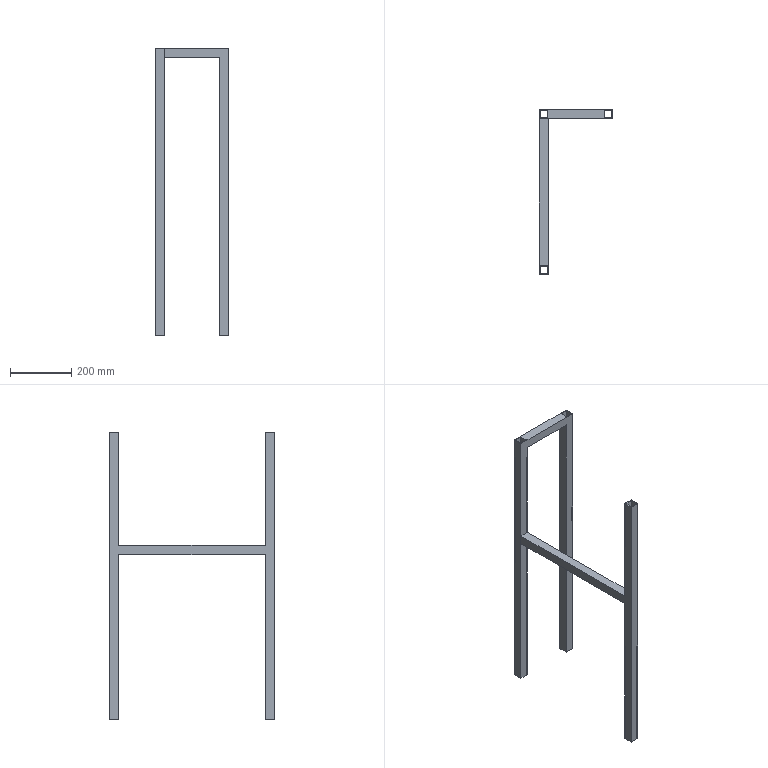Part | SolidWorks | features ICE 4, Extrusion 1 | 1 solid | 30 faces | box 240 x 540 x 940 mm | volume 1507680 mm3 | plane 30
STEP:
#1=CARTESIAN_POINT('',(213.,27.,0.));
#2=VERTEX_POINT('',#1);
#3=CARTESIAN_POINT('',(237.,27.,0.));
#4=VERTEX_POINT('',#3);
#5=CARTESIAN_POINT('',(0.,27.,0.));
#6=DIRECTION('',(1.,0.,0.));
#7=VECTOR('',#6,1000.);
#8=LINE('',#5,#7);
#9=EDGE_CURVE('',#2,#4,#8,.T.);
#10=ORIENTED_EDGE('',*,*,#9,.T.);
#11=CARTESIAN_POINT('',(237.,27.,940.));
#12=VERTEX_POINT('',#11);
#13=CARTESIAN_POINT('',(237.,27.,940.));
#14=DIRECTION('',(0.,0.,-1.));
#15=VECTOR('',#14,1000.);
#16=LINE('',#13,#15);
#17=EDGE_CURVE('',#12,#4,#16,.T.);
#18=ORIENTED_EDGE('',*,*,#17,.F.);
#19=CARTESIAN_POINT('',(213.,27.,940.));
#20=VERTEX_POINT('',#19);
#21=CARTESIAN_POINT('',(0.,27.,940.));
#22=DIRECTION('',(1.,0.,0.));
#23=VECTOR('',#22,1000.);
#24=LINE('',#21,#23);
#25=EDGE_CURVE('',#20,#12,#24,.T.);
#26=ORIENTED_EDGE('',*,*,#25,.F.);
#27=CARTESIAN_POINT('',(213.,27.,940.));
#28=DIRECTION('',(0.,0.,-1.));
#29=VECTOR('',#28,1000.);
#30=LINE('',#27,#29);
#31=EDGE_CURVE('',#20,#2,#30,.T.);
#32=ORIENTED_EDGE('',*,*,#31,.T.);
#33=EDGE_LOOP('',(#10,#18,#26,#32));
#34=FACE_OUTER_BOUND('',#33,.T.);
#35=CARTESIAN_POINT('',(0.,27.,940.));
#36=DIRECTION('',(0.,1.,0.));
#37=DIRECTION('',(0.,0.,1.));
#38=AXIS2_PLACEMENT_3D('',#35,#36,#37);
#39=PLANE('',#38);
#40=ADVANCED_FACE('',(#34),#39,.F.);
#41=CARTESIAN_POINT('',(237.,3.,0.));
#42=VERTEX_POINT('',#41);
#43=CARTESIAN_POINT('',(237.,0.,0.));
#44=DIRECTION('',(0.,-1.,0.));
#45=VECTOR('',#44,1000.);
#46=LINE('',#43,#45);
#47=EDGE_CURVE('',#4,#42,#46,.T.);
#48=ORIENTED_EDGE('',*,*,#47,.T.);
#49=CARTESIAN_POINT('',(237.,3.,940.));
#50=VERTEX_POINT('',#49);
#51=CARTESIAN_POINT('',(237.,3.,940.));
#52=DIRECTION('',(0.,0.,-1.));
#53=VECTOR('',#52,1000.);
#54=LINE('',#51,#53);
#55=EDGE_CURVE('',#50,#42,#54,.T.);
#56=ORIENTED_EDGE('',*,*,#55,.F.);
#57=CARTESIAN_POINT('',(237.,0.,940.));
#58=DIRECTION('',(0.,-1.,0.));
#59=VECTOR('',#58,1000.);
#60=LINE('',#57,#59);
#61=EDGE_CURVE('',#12,#50,#60,.T.);
#62=ORIENTED_EDGE('',*,*,#61,.F.);
#63=ORIENTED_EDGE('',*,*,#17,.T.);
#64=EDGE_LOOP('',(#48,#56,#62,#63));
#65=FACE_OUTER_BOUND('',#64,.T.);
#66=CARTESIAN_POINT('',(237.,0.,940.));
#67=DIRECTION('',(1.,0.,0.));
#68=DIRECTION('',(0.,0.,-1.));
#69=AXIS2_PLACEMENT_3D('',#66,#67,#68);
#70=PLANE('',#69);
#71=ADVANCED_FACE('',(#65),#70,.F.);
#72=CARTESIAN_POINT('',(213.,3.,0.));
#73=VERTEX_POINT('',#72);
#74=CARTESIAN_POINT('',(0.,3.,0.));
#75=DIRECTION('',(-1.,0.,0.));
#76=VECTOR('',#75,1000.);
#77=LINE('',#74,#76);
#78=EDGE_CURVE('',#42,#73,#77,.T.);
#79=ORIENTED_EDGE('',*,*,#78,.T.);
#80=CARTESIAN_POINT('',(213.,3.,940.));
#81=VERTEX_POINT('',#80);
#82=CARTESIAN_POINT('',(213.,3.,940.));
#83=DIRECTION('',(0.,0.,-1.));
#84=VECTOR('',#83,1000.);
#85=LINE('',#82,#84);
#86=EDGE_CURVE('',#81,#73,#85,.T.);
#87=ORIENTED_EDGE('',*,*,#86,.F.);
#88=CARTESIAN_POINT('',(0.,3.,940.));
#89=DIRECTION('',(-1.,0.,0.));
#90=VECTOR('',#89,1000.);
#91=LINE('',#88,#90);
#92=EDGE_CURVE('',#50,#81,#91,.T.);
#93=ORIENTED_EDGE('',*,*,#92,.F.);
#94=ORIENTED_EDGE('',*,*,#55,.T.);
#95=EDGE_LOOP('',(#79,#87,#93,#94));
#96=FACE_OUTER_BOUND('',#95,.T.);
#97=CARTESIAN_POINT('',(0.,3.,940.));
#98=DIRECTION('',(0.,-1.,0.));
#99=DIRECTION('',(0.,0.,-1.));
#100=AXIS2_PLACEMENT_3D('',#97,#98,#99);
#101=PLANE('',#100);
#102=ADVANCED_FACE('',(#96),#101,.F.);
#103=CARTESIAN_POINT('',(240.,0.,0.));
#104=VERTEX_POINT('',#103);
#105=CARTESIAN_POINT('',(210.,0.,0.));
#106=VERTEX_POINT('',#105);
#107=CARTESIAN_POINT('',(0.,0.,0.));
#108=DIRECTION('',(-1.,0.,0.));
#109=VECTOR('',#108,1000.);
#110=LINE('',#107,#109);
#111=EDGE_CURVE('',#104,#106,#110,.T.);
#112=ORIENTED_EDGE('',*,*,#111,.F.);
#113=CARTESIAN_POINT('',(240.,0.,940.));
#114=VERTEX_POINT('',#113);
#115=CARTESIAN_POINT('',(240.,0.,940.));
#116=DIRECTION('',(0.,0.,-1.));
#117=VECTOR('',#116,1000.);
#118=LINE('',#115,#117);
#119=EDGE_CURVE('',#114,#104,#118,.T.);
#120=ORIENTED_EDGE('',*,*,#119,.F.);
#121=CARTESIAN_POINT('',(0.,0.,940.));
#122=VERTEX_POINT('',#121);
#123=CARTESIAN_POINT('',(0.,0.,940.));
#124=DIRECTION('',(-1.,0.,0.));
#125=VECTOR('',#124,1000.);
#126=LINE('',#123,#125);
#127=EDGE_CURVE('',#114,#122,#126,.T.);
#128=ORIENTED_EDGE('',*,*,#127,.T.);
#129=CARTESIAN_POINT('',(0.,0.,570.));
#130=VERTEX_POINT('',#129);
#131=CARTESIAN_POINT('',(0.,0.,940.));
#132=DIRECTION('',(0.,0.,-1.));
#133=VECTOR('',#132,1000.);
#134=LINE('',#131,#133);
#135=EDGE_CURVE('',#122,#130,#134,.T.);
#136=ORIENTED_EDGE('',*,*,#135,.T.);
#137=CARTESIAN_POINT('',(30.,0.,570.));
#138=VERTEX_POINT('',#137);
#139=CARTESIAN_POINT('',(30.,0.,570.));
#140=DIRECTION('',(-1.,0.,0.));
#141=VECTOR('',#140,1000.);
#142=LINE('',#139,#141);
#143=EDGE_CURVE('',#138,#130,#142,.T.);
#144=ORIENTED_EDGE('',*,*,#143,.F.);
#145=CARTESIAN_POINT('',(30.,0.,910.));
#146=VERTEX_POINT('',#145);
#147=CARTESIAN_POINT('',(30.,0.,940.));
#148=DIRECTION('',(0.,0.,-1.));
#149=VECTOR('',#148,1000.);
#150=LINE('',#147,#149);
#151=EDGE_CURVE('',#146,#138,#150,.T.);
#152=ORIENTED_EDGE('',*,*,#151,.F.);
#153=CARTESIAN_POINT('',(210.,0.,910.));
#154=VERTEX_POINT('',#153);
#155=CARTESIAN_POINT('',(30.,0.,910.));
#156=DIRECTION('',(1.,0.,0.));
#157=VECTOR('',#156,1000.);
#158=LINE('',#155,#157);
#159=EDGE_CURVE('',#146,#154,#158,.T.);
#160=ORIENTED_EDGE('',*,*,#159,.T.);
#161=CARTESIAN_POINT('',(210.,0.,940.));
#162=DIRECTION('',(0.,0.,-1.));
#163=VECTOR('',#162,1000.);
#164=LINE('',#161,#163);
#165=EDGE_CURVE('',#154,#106,#164,.T.);
#166=ORIENTED_EDGE('',*,*,#165,.T.);
#167=EDGE_LOOP('',(#112,#120,#128,#136,#144,#152,#160,#166));
#168=FACE_OUTER_BOUND('',#167,.T.);
#169=CARTESIAN_POINT('',(0.,0.,940.));
#170=DIRECTION('',(0.,-1.,0.));
#171=DIRECTION('',(0.,0.,-1.));
#172=AXIS2_PLACEMENT_3D('',#169,#170,#171);
#173=PLANE('',#172);
#174=ADVANCED_FACE('',(#168),#173,.T.);
#175=CARTESIAN_POINT('',(240.,30.,0.));
#176=VERTEX_POINT('',#175);
#177=CARTESIAN_POINT('',(240.,0.,0.));
#178=DIRECTION('',(0.,-1.,0.));
#179=VECTOR('',#178,1000.);
#180=LINE('',#177,#179);
#181=EDGE_CURVE('',#176,#104,#180,.T.);
#182=ORIENTED_EDGE('',*,*,#181,.F.);
#183=CARTESIAN_POINT('',(240.,30.,940.));
#184=VERTEX_POINT('',#183);
#185=CARTESIAN_POINT('',(240.,30.,940.));
#186=DIRECTION('',(0.,0.,-1.));
#187=VECTOR('',#186,1000.);
#188=LINE('',#185,#187);
#189=EDGE_CURVE('',#184,#176,#188,.T.);
#190=ORIENTED_EDGE('',*,*,#189,.F.);
#191=CARTESIAN_POINT('',(240.,0.,940.));
#192=DIRECTION('',(0.,-1.,0.));
#193=VECTOR('',#192,1000.);
#194=LINE('',#191,#193);
#195=EDGE_CURVE('',#184,#114,#194,.T.);
#196=ORIENTED_EDGE('',*,*,#195,.T.);
#197=ORIENTED_EDGE('',*,*,#119,.T.);
#198=EDGE_LOOP('',(#182,#190,#196,#197));
#199=FACE_OUTER_BOUND('',#198,.T.);
#200=CARTESIAN_POINT('',(240.,0.,940.));
#201=DIRECTION('',(1.,0.,0.));
#202=DIRECTION('',(0.,0.,-1.));
#203=AXIS2_PLACEMENT_3D('',#200,#201,#202);
#204=PLANE('',#203);
#205=ADVANCED_FACE('',(#199),#204,.T.);
#206=CARTESIAN_POINT('',(210.,30.,0.));
#207=VERTEX_POINT('',#206);
#208=CARTESIAN_POINT('',(0.,30.,0.));
#209=DIRECTION('',(1.,0.,0.));
#210=VECTOR('',#209,1000.);
#211=LINE('',#208,#210);
#212=EDGE_CURVE('',#207,#176,#211,.T.);
#213=ORIENTED_EDGE('',*,*,#212,.F.);
#214=CARTESIAN_POINT('',(210.,30.,910.));
#215=VERTEX_POINT('',#214);
#216=CARTESIAN_POINT('',(210.,30.,940.));
#217=DIRECTION('',(0.,0.,-1.));
#218=VECTOR('',#217,1000.);
#219=LINE('',#216,#218);
#220=EDGE_CURVE('',#215,#207,#219,.T.);
#221=ORIENTED_EDGE('',*,*,#220,.F.);
#222=CARTESIAN_POINT('',(30.,30.,910.));
#223=VERTEX_POINT('',#222);
#224=CARTESIAN_POINT('',(30.,30.,910.));
#225=DIRECTION('',(1.,0.,0.));
#226=VECTOR('',#225,1000.);
#227=LINE('',#224,#226);
#228=EDGE_CURVE('',#223,#215,#227,.T.);
#229=ORIENTED_EDGE('',*,*,#228,.F.);
#230=CARTESIAN_POINT('',(30.,30.,0.));
#231=VERTEX_POINT('',#230);
#232=CARTESIAN_POINT('',(30.,30.,940.));
#233=DIRECTION('',(0.,0.,-1.));
#234=VECTOR('',#233,1000.);
#235=LINE('',#232,#234);
#236=EDGE_CURVE('',#223,#231,#235,.T.);
#237=ORIENTED_EDGE('',*,*,#236,.T.);
#238=CARTESIAN_POINT('',(0.,30.,0.));
#239=VERTEX_POINT('',#238);
#240=CARTESIAN_POINT('',(0.,30.,0.));
#241=DIRECTION('',(1.,0.,0.));
#242=VECTOR('',#241,1000.);
#243=LINE('',#240,#242);
#244=EDGE_CURVE('',#239,#231,#243,.T.);
#245=ORIENTED_EDGE('',*,*,#244,.F.);
#246=CARTESIAN_POINT('',(0.,30.,940.));
#247=VERTEX_POINT('',#246);
#248=CARTESIAN_POINT('',(0.,30.,940.));
#249=DIRECTION('',(0.,0.,-1.));
#250=VECTOR('',#249,1000.);
#251=LINE('',#248,#250);
#252=EDGE_CURVE('',#247,#239,#251,.T.);
#253=ORIENTED_EDGE('',*,*,#252,.F.);
#254=CARTESIAN_POINT('',(0.,30.,940.));
#255=DIRECTION('',(1.,0.,0.));
#256=VECTOR('',#255,1000.);
#257=LINE('',#254,#256);
#258=EDGE_CURVE('',#247,#184,#257,.T.);
#259=ORIENTED_EDGE('',*,*,#258,.T.);
#260=ORIENTED_EDGE('',*,*,#189,.T.);
#261=EDGE_LOOP('',(#213,#221,#229,#237,#245,#253,#259,#260));
#262=FACE_OUTER_BOUND('',#261,.T.);
#263=CARTESIAN_POINT('',(0.,30.,940.));
#264=DIRECTION('',(0.,1.,0.));
#265=DIRECTION('',(0.,0.,1.));
#266=AXIS2_PLACEMENT_3D('',#263,#264,#265);
#267=PLANE('',#266);
#268=ADVANCED_FACE('',(#262),#267,.T.);
#269=CARTESIAN_POINT('',(210.,30.,910.));
#270=DIRECTION('',(0.,-1.,0.));
#271=VECTOR('',#270,1000.);
#272=LINE('',#269,#271);
#273=EDGE_CURVE('',#215,#154,#272,.T.);
#274=ORIENTED_EDGE('',*,*,#273,.F.);
#275=ORIENTED_EDGE('',*,*,#220,.T.);
#276=CARTESIAN_POINT('',(210.,0.,0.));
#277=DIRECTION('',(0.,1.,0.));
#278=VECTOR('',#277,1000.);
#279=LINE('',#276,#278);
#280=EDGE_CURVE('',#106,#207,#279,.T.);
#281=ORIENTED_EDGE('',*,*,#280,.F.);
#282=ORIENTED_EDGE('',*,*,#165,.F.);
#283=EDGE_LOOP('',(#274,#275,#281,#282));
#284=FACE_OUTER_BOUND('',#283,.T.);
#285=CARTESIAN_POINT('',(210.,0.,940.));
#286=DIRECTION('',(-1.,0.,0.));
#287=DIRECTION('',(0.,0.,1.));
#288=AXIS2_PLACEMENT_3D('',#285,#286,#287);
#289=PLANE('',#288);
#290=ADVANCED_FACE('',(#284),#289,.T.);
#291=CARTESIAN_POINT('',(213.,0.,0.));
#292=DIRECTION('',(0.,1.,0.));
#293=VECTOR('',#292,1000.);
#294=LINE('',#291,#293);
#295=EDGE_CURVE('',#73,#2,#294,.T.);
#296=ORIENTED_EDGE('',*,*,#295,.T.);
#297=ORIENTED_EDGE('',*,*,#31,.F.);
#298=CARTESIAN_POINT('',(213.,0.,940.));
#299=DIRECTION('',(0.,1.,0.));
#300=VECTOR('',#299,1000.);
#301=LINE('',#298,#300);
#302=EDGE_CURVE('',#81,#20,#301,.T.);
#303=ORIENTED_EDGE('',*,*,#302,.F.);
#304=ORIENTED_EDGE('',*,*,#86,.T.);
#305=EDGE_LOOP('',(#296,#297,#303,#304));
#306=FACE_OUTER_BOUND('',#305,.T.);
#307=CARTESIAN_POINT('',(213.,0.,940.));
#308=DIRECTION('',(-1.,0.,0.));
#309=DIRECTION('',(0.,0.,1.));
#310=AXIS2_PLACEMENT_3D('',#307,#308,#309);
#311=PLANE('',#310);
#312=ADVANCED_FACE('',(#306),#311,.F.);
#313=ORIENTED_EDGE('',*,*,#127,.F.);
#314=ORIENTED_EDGE('',*,*,#195,.F.);
#315=ORIENTED_EDGE('',*,*,#258,.F.);
#316=CARTESIAN_POINT('',(0.,0.,940.));
#317=DIRECTION('',(0.,1.,0.));
#318=VECTOR('',#317,1000.);
#319=LINE('',#316,#318);
#320=EDGE_CURVE('',#122,#247,#319,.T.);
#321=ORIENTED_EDGE('',*,*,#320,.F.);
#322=EDGE_LOOP('',(#313,#314,#315,#321));
#323=FACE_OUTER_BOUND('',#322,.T.);
#324=ORIENTED_EDGE('',*,*,#25,.T.);
#325=ORIENTED_EDGE('',*,*,#61,.T.);
#326=ORIENTED_EDGE('',*,*,#92,.T.);
#327=ORIENTED_EDGE('',*,*,#302,.T.);
#328=EDGE_LOOP('',(#324,#325,#326,#327));
#329=FACE_BOUND('',#328,.T.);
#330=CARTESIAN_POINT('',(27.,27.,940.));
#331=VERTEX_POINT('',#330);
#332=CARTESIAN_POINT('',(27.,3.,940.));
#333=VERTEX_POINT('',#332);
#334=CARTESIAN_POINT('',(27.,0.,940.));
#335=DIRECTION('',(0.,-1.,0.));
#336=VECTOR('',#335,1000.);
#337=LINE('',#334,#336);
#338=EDGE_CURVE('',#331,#333,#337,.T.);
#339=ORIENTED_EDGE('',*,*,#338,.T.);
#340=CARTESIAN_POINT('',(3.,3.,940.));
#341=VERTEX_POINT('',#340);
#342=CARTESIAN_POINT('',(0.,3.,940.));
#343=DIRECTION('',(-1.,0.,0.));
#344=VECTOR('',#343,1000.);
#345=LINE('',#342,#344);
#346=EDGE_CURVE('',#333,#341,#345,.T.);
#347=ORIENTED_EDGE('',*,*,#346,.T.);
#348=CARTESIAN_POINT('',(3.,27.,940.));
#349=VERTEX_POINT('',#348);
#350=CARTESIAN_POINT('',(3.,0.,940.));
#351=DIRECTION('',(0.,1.,0.));
#352=VECTOR('',#351,1000.);
#353=LINE('',#350,#352);
#354=EDGE_CURVE('',#341,#349,#353,.T.);
#355=ORIENTED_EDGE('',*,*,#354,.T.);
#356=CARTESIAN_POINT('',(0.,27.,940.));
#357=DIRECTION('',(1.,0.,0.));
#358=VECTOR('',#357,1000.);
#359=LINE('',#356,#358);
#360=EDGE_CURVE('',#349,#331,#359,.T.);
#361=ORIENTED_EDGE('',*,*,#360,.T.);
#362=EDGE_LOOP('',(#339,#347,#355,#361));
#363=FACE_BOUND('',#362,.T.);
#364=CARTESIAN_POINT('',(0.,0.,940.));
#365=DIRECTION('',(0.,0.,1.));
#366=DIRECTION('',(1.,0.,0.));
#367=AXIS2_PLACEMENT_3D('',#364,#365,#366);
#368=PLANE('',#367);
#369=ADVANCED_FACE('',(#323,#329,#363),#368,.T.);
#370=ORIENTED_EDGE('',*,*,#111,.T.);
#371=ORIENTED_EDGE('',*,*,#280,.T.);
#372=ORIENTED_EDGE('',*,*,#212,.T.);
#373=ORIENTED_EDGE('',*,*,#181,.T.);
#374=EDGE_LOOP('',(#370,#371,#372,#373));
#375=FACE_OUTER_BOUND('',#374,.T.);
#376=ORIENTED_EDGE('',*,*,#9,.F.);
#377=ORIENTED_EDGE('',*,*,#295,.F.);
#378=ORIENTED_EDGE('',*,*,#78,.F.);
#379=ORIENTED_EDGE('',*,*,#47,.F.);
#380=EDGE_LOOP('',(#376,#377,#378,#379));
#381=FACE_BOUND('',#380,.T.);
#382=CARTESIAN_POINT('',(0.,0.,0.));
#383=DIRECTION('',(0.,0.,1.));
#384=DIRECTION('',(1.,0.,0.));
#385=AXIS2_PLACEMENT_3D('',#382,#383,#384);
#386=PLANE('',#385);
#387=ADVANCED_FACE('',(#375,#381),#386,.F.);
#388=ORIENTED_EDGE('',*,*,#273,.T.);
#389=ORIENTED_EDGE('',*,*,#159,.F.);
#390=CARTESIAN_POINT('',(30.,30.,910.));
#391=DIRECTION('',(0.,-1.,0.));
#392=VECTOR('',#391,1000.);
#393=LINE('',#390,#392);
#394=EDGE_CURVE('',#223,#146,#393,.T.);
#395=ORIENTED_EDGE('',*,*,#394,.F.);
#396=ORIENTED_EDGE('',*,*,#228,.T.);
#397=EDGE_LOOP('',(#388,#389,#395,#396));
#398=FACE_OUTER_BOUND('',#397,.T.);
#399=CARTESIAN_POINT('',(30.,30.,910.));
#400=DIRECTION('',(0.,0.,1.));
#401=DIRECTION('',(1.,0.,0.));
#402=AXIS2_PLACEMENT_3D('',#399,#400,#401);
#403=PLANE('',#402);
#404=ADVANCED_FACE('',(#398),#403,.F.);
#405=CARTESIAN_POINT('',(30.,0.,540.));
#406=VERTEX_POINT('',#405);
#407=CARTESIAN_POINT('',(30.,0.,0.));
#408=VERTEX_POINT('',#407);
#409=CARTESIAN_POINT('',(30.,0.,940.));
#410=DIRECTION('',(0.,0.,-1.));
#411=VECTOR('',#410,1000.);
#412=LINE('',#409,#411);
#413=EDGE_CURVE('',#406,#408,#412,.T.);
#414=ORIENTED_EDGE('',*,*,#413,.F.);
#415=CARTESIAN_POINT('',(0.,0.,540.));
#416=VERTEX_POINT('',#415);
#417=CARTESIAN_POINT('',(30.,0.,540.));
#418=DIRECTION('',(-1.,0.,0.));
#419=VECTOR('',#418,1000.);
#420=LINE('',#417,#419);
#421=EDGE_CURVE('',#406,#416,#420,.T.);
#422=ORIENTED_EDGE('',*,*,#421,.T.);
#423=CARTESIAN_POINT('',(0.,0.,0.));
#424=VERTEX_POINT('',#423);
#425=CARTESIAN_POINT('',(0.,0.,940.));
#426=DIRECTION('',(0.,0.,-1.));
#427=VECTOR('',#426,1000.);
#428=LINE('',#425,#427);
#429=EDGE_CURVE('',#416,#424,#428,.T.);
#430=ORIENTED_EDGE('',*,*,#429,.T.);
#431=CARTESIAN_POINT('',(0.,0.,0.));
#432=DIRECTION('',(-1.,0.,0.));
#433=VECTOR('',#432,1000.);
#434=LINE('',#431,#433);
#435=EDGE_CURVE('',#408,#424,#434,.T.);
#436=ORIENTED_EDGE('',*,*,#435,.F.);
#437=EDGE_LOOP('',(#414,#422,#430,#436));
#438=FACE_OUTER_BOUND('',#437,.T.);
#439=CARTESIAN_POINT('',(0.,0.,940.));
#440=DIRECTION('',(0.,-1.,0.));
#441=DIRECTION('',(0.,0.,-1.));
#442=AXIS2_PLACEMENT_3D('',#439,#440,#441);
#443=PLANE('',#442);
#444=ADVANCED_FACE('',(#438),#443,.T.);
#445=ORIENTED_EDGE('',*,*,#236,.F.);
#446=ORIENTED_EDGE('',*,*,#394,.T.);
#447=ORIENTED_EDGE('',*,*,#151,.T.);
#448=CARTESIAN_POINT('',(30.,-480.,570.));
#449=VERTEX_POINT('',#448);
#450=CARTESIAN_POINT('',(30.,0.,570.));
#451=DIRECTION('',(0.,1.,0.));
#452=VECTOR('',#451,1000.);
#453=LINE('',#450,#452);
#454=EDGE_CURVE('',#449,#138,#453,.T.);
#455=ORIENTED_EDGE('',*,*,#454,.F.);
#456=CARTESIAN_POINT('',(30.,-480.,940.));
#457=VERTEX_POINT('',#456);
#458=CARTESIAN_POINT('',(30.,-480.,940.));
#459=DIRECTION('',(0.,0.,-1.));
#460=VECTOR('',#459,1000.);
#461=LINE('',#458,#460);
#462=EDGE_CURVE('',#457,#449,#461,.T.);
#463=ORIENTED_EDGE('',*,*,#462,.F.);
#464=CARTESIAN_POINT('',(30.,-510.,940.));
#465=VERTEX_POINT('',#464);
#466=CARTESIAN_POINT('',(30.,0.,940.));
#467=DIRECTION('',(0.,-1.,0.));
#468=VECTOR('',#467,1000.);
#469=LINE('',#466,#468);
#470=EDGE_CURVE('',#457,#465,#469,.T.);
#471=ORIENTED_EDGE('',*,*,#470,.T.);
#472=CARTESIAN_POINT('',(30.,-510.,0.));
#473=VERTEX_POINT('',#472);
#474=CARTESIAN_POINT('',(30.,-510.,940.));
#475=DIRECTION('',(0.,0.,-1.));
#476=VECTOR('',#475,1000.);
#477=LINE('',#474,#476);
#478=EDGE_CURVE('',#465,#473,#477,.T.);
#479=ORIENTED_EDGE('',*,*,#478,.T.);
#480=CARTESIAN_POINT('',(30.,-480.,0.));
#481=VERTEX_POINT('',#480);
#482=CARTESIAN_POINT('',(30.,0.,0.));
#483=DIRECTION('',(0.,-1.,0.));
#484=VECTOR('',#483,1000.);
#485=LINE('',#482,#484);
#486=EDGE_CURVE('',#481,#473,#485,.T.);
#487=ORIENTED_EDGE('',*,*,#486,.F.);
#488=CARTESIAN_POINT('',(30.,-480.,540.));
#489=VERTEX_POINT('',#488);
#490=CARTESIAN_POINT('',(30.,-480.,940.));
#491=DIRECTION('',(0.,0.,-1.));
#492=VECTOR('',#491,1000.);
#493=LINE('',#490,#492);
#494=EDGE_CURVE('',#489,#481,#493,.T.);
#495=ORIENTED_EDGE('',*,*,#494,.F.);
#496=CARTESIAN_POINT('',(30.,0.,540.));
#497=DIRECTION('',(0.,-1.,0.));
#498=VECTOR('',#497,1000.);
#499=LINE('',#496,#498);
#500=EDGE_CURVE('',#406,#489,#499,.T.);
#501=ORIENTED_EDGE('',*,*,#500,.F.);
#502=ORIENTED_EDGE('',*,*,#413,.T.);
#503=CARTESIAN_POINT('',(30.,0.,0.));
#504=DIRECTION('',(0.,-1.,0.));
#505=VECTOR('',#504,1000.);
#506=LINE('',#503,#505);
#507=EDGE_CURVE('',#231,#408,#506,.T.);
#508=ORIENTED_EDGE('',*,*,#507,.F.);
#509=EDGE_LOOP('',(#445,#446,#447,#455,#463,#471,#479,#487,#495,#501,#502,#508));
#510=FACE_OUTER_BOUND('',#509,.T.);
#511=CARTESIAN_POINT('',(30.,0.,940.));
#512=DIRECTION('',(1.,0.,0.));
#513=DIRECTION('',(0.,0.,-1.));
#514=AXIS2_PLACEMENT_3D('',#511,#512,#513);
#515=PLANE('',#514);
#516=ADVANCED_FACE('',(#510),#515,.T.);
#517=ORIENTED_EDGE('',*,*,#135,.F.);
#518=ORIENTED_EDGE('',*,*,#320,.T.);
#519=ORIENTED_EDGE('',*,*,#252,.T.);
#520=CARTESIAN_POINT('',(0.,0.,0.));
#521=DIRECTION('',(0.,1.,0.));
#522=VECTOR('',#521,1000.);
#523=LINE('',#520,#522);
#524=EDGE_CURVE('',#424,#239,#523,.T.);
#525=ORIENTED_EDGE('',*,*,#524,.F.);
#526=ORIENTED_EDGE('',*,*,#429,.F.);
#527=CARTESIAN_POINT('',(0.,-480.,540.));
#528=VERTEX_POINT('',#527);
#529=CARTESIAN_POINT('',(0.,0.,540.));
#530=DIRECTION('',(0.,-1.,0.));
#531=VECTOR('',#530,1000.);
#532=LINE('',#529,#531);
#533=EDGE_CURVE('',#416,#528,#532,.T.);
#534=ORIENTED_EDGE('',*,*,#533,.T.);
#535=CARTESIAN_POINT('',(0.,-480.,0.));
#536=VERTEX_POINT('',#535);
#537=CARTESIAN_POINT('',(0.,-480.,940.));
#538=DIRECTION('',(0.,0.,-1.));
#539=VECTOR('',#538,1000.);
#540=LINE('',#537,#539);
#541=EDGE_CURVE('',#528,#536,#540,.T.);
#542=ORIENTED_EDGE('',*,*,#541,.T.);
#543=CARTESIAN_POINT('',(0.,-510.,0.));
#544=VERTEX_POINT('',#543);
#545=CARTESIAN_POINT('',(0.,0.,0.));
#546=DIRECTION('',(0.,-1.,0.));
#547=VECTOR('',#546,1000.);
#548=LINE('',#545,#547);
#549=EDGE_CURVE('',#536,#544,#548,.T.);
#550=ORIENTED_EDGE('',*,*,#549,.T.);
#551=CARTESIAN_POINT('',(0.,-510.,940.));
#552=VERTEX_POINT('',#551);
#553=CARTESIAN_POINT('',(0.,-510.,940.));
#554=DIRECTION('',(0.,0.,-1.));
#555=VECTOR('',#554,1000.);
#556=LINE('',#553,#555);
#557=EDGE_CURVE('',#552,#544,#556,.T.);
#558=ORIENTED_EDGE('',*,*,#557,.F.);
#559=CARTESIAN_POINT('',(0.,-480.,940.));
#560=VERTEX_POINT('',#559);
#561=CARTESIAN_POINT('',(0.,0.,940.));
#562=DIRECTION('',(0.,-1.,0.));
#563=VECTOR('',#562,1000.);
#564=LINE('',#561,#563);
#565=EDGE_CURVE('',#560,#552,#564,.T.);
#566=ORIENTED_EDGE('',*,*,#565,.F.);
#567=CARTESIAN_POINT('',(0.,-480.,570.));
#568=VERTEX_POINT('',#567);
#569=CARTESIAN_POINT('',(0.,-480.,940.));
#570=DIRECTION('',(0.,0.,-1.));
#571=VECTOR('',#570,1000.);
#572=LINE('',#569,#571);
#573=EDGE_CURVE('',#560,#568,#572,.T.);
#574=ORIENTED_EDGE('',*,*,#573,.T.);
#575=CARTESIAN_POINT('',(0.,0.,570.));
#576=DIRECTION('',(0.,1.,0.));
#577=VECTOR('',#576,1000.);
#578=LINE('',#575,#577);
#579=EDGE_CURVE('',#568,#130,#578,.T.);
#580=ORIENTED_EDGE('',*,*,#579,.T.);
#581=EDGE_LOOP('',(#517,#518,#519,#525,#526,#534,#542,#550,#558,#566,#574,#580));
#582=FACE_OUTER_BOUND('',#581,.T.);
#583=CARTESIAN_POINT('',(0.,0.,940.));
#584=DIRECTION('',(-1.,0.,0.));
#585=DIRECTION('',(0.,0.,1.));
#586=AXIS2_PLACEMENT_3D('',#583,#584,#585);
#587=PLANE('',#586);
#588=ADVANCED_FACE('',(#582),#587,.T.);
#589=CARTESIAN_POINT('',(27.,27.,0.));
#590=VERTEX_POINT('',#589);
#591=CARTESIAN_POINT('',(27.,3.,0.));
#592=VERTEX_POINT('',#591);
#593=CARTESIAN_POINT('',(27.,0.,0.));
#594=DIRECTION('',(0.,-1.,0.));
#595=VECTOR('',#594,1000.);
#596=LINE('',#593,#595);
#597=EDGE_CURVE('',#590,#592,#596,.T.);
#598=ORIENTED_EDGE('',*,*,#597,.T.);
#599=CARTESIAN_POINT('',(27.,3.,940.));
#600=DIRECTION('',(0.,0.,-1.));
#601=VECTOR('',#600,1000.);
#602=LINE('',#599,#601);
#603=EDGE_CURVE('',#333,#592,#602,.T.);
#604=ORIENTED_EDGE('',*,*,#603,.F.);
#605=ORIENTED_EDGE('',*,*,#338,.F.);
#606=CARTESIAN_POINT('',(27.,27.,940.));
#607=DIRECTION('',(0.,0.,-1.));
#608=VECTOR('',#607,1000.);
#609=LINE('',#606,#608);
#610=EDGE_CURVE('',#331,#590,#609,.T.);
#611=ORIENTED_EDGE('',*,*,#610,.T.);
#612=EDGE_LOOP('',(#598,#604,#605,#611));
#613=FACE_OUTER_BOUND('',#612,.T.);
#614=CARTESIAN_POINT('',(27.,0.,940.));
#615=DIRECTION('',(1.,0.,0.));
#616=DIRECTION('',(0.,0.,-1.));
#617=AXIS2_PLACEMENT_3D('',#614,#615,#616);
#618=PLANE('',#617);
#619=ADVANCED_FACE('',(#613),#618,.F.);
#620=CARTESIAN_POINT('',(3.,3.,0.));
#621=VERTEX_POINT('',#620);
#622=CARTESIAN_POINT('',(0.,3.,0.));
#623=DIRECTION('',(-1.,0.,0.));
#624=VECTOR('',#623,1000.);
#625=LINE('',#622,#624);
#626=EDGE_CURVE('',#592,#621,#625,.T.);
#627=ORIENTED_EDGE('',*,*,#626,.T.);
#628=CARTESIAN_POINT('',(3.,3.,940.));
#629=DIRECTION('',(0.,0.,-1.));
#630=VECTOR('',#629,1000.);
#631=LINE('',#628,#630);
#632=EDGE_CURVE('',#341,#621,#631,.T.);
#633=ORIENTED_EDGE('',*,*,#632,.F.);
#634=ORIENTED_EDGE('',*,*,#346,.F.);
#635=ORIENTED_EDGE('',*,*,#603,.T.);
#636=EDGE_LOOP('',(#627,#633,#634,#635));
#637=FACE_OUTER_BOUND('',#636,.T.);
#638=CARTESIAN_POINT('',(0.,3.,940.));
#639=DIRECTION('',(0.,-1.,0.));
#640=DIRECTION('',(0.,0.,-1.));
#641=AXIS2_PLACEMENT_3D('',#638,#639,#640);
#642=PLANE('',#641);
#643=ADVANCED_FACE('',(#637),#642,.F.);
#644=CARTESIAN_POINT('',(3.,27.,0.));
#645=VERTEX_POINT('',#644);
#646=CARTESIAN_POINT('',(3.,0.,0.));
#647=DIRECTION('',(0.,1.,0.));
#648=VECTOR('',#647,1000.);
#649=LINE('',#646,#648);
#650=EDGE_CURVE('',#621,#645,#649,.T.);
#651=ORIENTED_EDGE('',*,*,#650,.T.);
#652=CARTESIAN_POINT('',(3.,27.,940.));
#653=DIRECTION('',(0.,0.,-1.));
#654=VECTOR('',#653,1000.);
#655=LINE('',#652,#654);
#656=EDGE_CURVE('',#349,#645,#655,.T.);
#657=ORIENTED_EDGE('',*,*,#656,.F.);
#658=ORIENTED_EDGE('',*,*,#354,.F.);
#659=ORIENTED_EDGE('',*,*,#632,.T.);
#660=EDGE_LOOP('',(#651,#657,#658,#659));
#661=FACE_OUTER_BOUND('',#660,.T.);
#662=CARTESIAN_POINT('',(3.,0.,940.));
#663=DIRECTION('',(-1.,0.,0.));
#664=DIRECTION('',(0.,0.,1.));
#665=AXIS2_PLACEMENT_3D('',#662,#663,#664);
#666=PLANE('',#665);
#667=ADVANCED_FACE('',(#661),#666,.F.);
#668=CARTESIAN_POINT('',(0.,27.,0.));
#669=DIRECTION('',(1.,0.,0.));
#670=VECTOR('',#669,1000.);
#671=LINE('',#668,#670);
#672=EDGE_CURVE('',#645,#590,#671,.T.);
#673=ORIENTED_EDGE('',*,*,#672,.T.);
#674=ORIENTED_EDGE('',*,*,#610,.F.);
#675=ORIENTED_EDGE('',*,*,#360,.F.);
#676=ORIENTED_EDGE('',*,*,#656,.T.);
#677=EDGE_LOOP('',(#673,#674,#675,#676));
#678=FACE_OUTER_BOUND('',#677,.T.);
#679=CARTESIAN_POINT('',(0.,27.,940.));
#680=DIRECTION('',(0.,1.,0.));
#681=DIRECTION('',(0.,0.,1.));
#682=AXIS2_PLACEMENT_3D('',#679,#680,#681);
#683=PLANE('',#682);
#684=ADVANCED_FACE('',(#678),#683,.F.);
#685=ORIENTED_EDGE('',*,*,#435,.T.);
#686=ORIENTED_EDGE('',*,*,#524,.T.);
#687=ORIENTED_EDGE('',*,*,#244,.T.);
#688=ORIENTED_EDGE('',*,*,#507,.T.);
#689=EDGE_LOOP('',(#685,#686,#687,#688));
#690=FACE_OUTER_BOUND('',#689,.T.);
#691=ORIENTED_EDGE('',*,*,#597,.F.);
#692=ORIENTED_EDGE('',*,*,#672,.F.);
#693=ORIENTED_EDGE('',*,*,#650,.F.);
#694=ORIENTED_EDGE('',*,*,#626,.F.);
#695=EDGE_LOOP('',(#691,#692,#693,#694));
#696=FACE_BOUND('',#695,.T.);
#697=CARTESIAN_POINT('',(0.,0.,0.));
#698=DIRECTION('',(0.,0.,1.));
#699=DIRECTION('',(1.,0.,0.));
#700=AXIS2_PLACEMENT_3D('',#697,#698,#699);
#701=PLANE('',#700);
#702=ADVANCED_FACE('',(#690,#696),#701,.F.);
#703=ORIENTED_EDGE('',*,*,#533,.F.);
#704=ORIENTED_EDGE('',*,*,#421,.F.);
#705=ORIENTED_EDGE('',*,*,#500,.T.);
#706=CARTESIAN_POINT('',(30.,-480.,540.));
#707=DIRECTION('',(-1.,0.,0.));
#708=VECTOR('',#707,1000.);
#709=LINE('',#706,#708);
#710=EDGE_CURVE('',#489,#528,#709,.T.);
#711=ORIENTED_EDGE('',*,*,#710,.T.);
#712=EDGE_LOOP('',(#703,#704,#705,#711));
#713=FACE_OUTER_BOUND('',#712,.T.);
#714=CARTESIAN_POINT('',(30.,0.,540.));
#715=DIRECTION('',(0.,0.,-1.));
#716=DIRECTION('',(-1.,0.,0.));
#717=AXIS2_PLACEMENT_3D('',#714,#715,#716);
#718=PLANE('',#717);
#719=ADVANCED_FACE('',(#713),#718,.T.);
#720=ORIENTED_EDGE('',*,*,#579,.F.);
#721=CARTESIAN_POINT('',(30.,-480.,570.));
#722=DIRECTION('',(-1.,0.,0.));
#723=VECTOR('',#722,1000.);
#724=LINE('',#721,#723);
#725=EDGE_CURVE('',#449,#568,#724,.T.);
#726=ORIENTED_EDGE('',*,*,#725,.F.);
#727=ORIENTED_EDGE('',*,*,#454,.T.);
#728=ORIENTED_EDGE('',*,*,#143,.T.);
#729=EDGE_LOOP('',(#720,#726,#727,#728));
#730=FACE_OUTER_BOUND('',#729,.T.);
#731=CARTESIAN_POINT('',(30.,0.,570.));
#732=DIRECTION('',(0.,0.,1.));
#733=DIRECTION('',(1.,0.,0.));
#734=AXIS2_PLACEMENT_3D('',#731,#732,#733);
#735=PLANE('',#734);
#736=ADVANCED_FACE('',(#730),#735,.T.);
#737=ORIENTED_EDGE('',*,*,#710,.F.);
#738=ORIENTED_EDGE('',*,*,#494,.T.);
#739=CARTESIAN_POINT('',(0.,-480.,0.));
#740=DIRECTION('',(1.,0.,0.));
#741=VECTOR('',#740,1000.);
#742=LINE('',#739,#741);
#743=EDGE_CURVE('',#536,#481,#742,.T.);
#744=ORIENTED_EDGE('',*,*,#743,.F.);
#745=ORIENTED_EDGE('',*,*,#541,.F.);
#746=EDGE_LOOP('',(#737,#738,#744,#745));
#747=FACE_OUTER_BOUND('',#746,.T.);
#748=CARTESIAN_POINT('',(0.,-480.,940.));
#749=DIRECTION('',(0.,1.,0.));
#750=DIRECTION('',(0.,0.,1.));
#751=AXIS2_PLACEMENT_3D('',#748,#749,#750);
#752=PLANE('',#751);
#753=ADVANCED_FACE('',(#747),#752,.T.);
#754=CARTESIAN_POINT('',(27.,-507.,0.));
#755=VERTEX_POINT('',#754);
#756=CARTESIAN_POINT('',(3.,-507.,0.));
#757=VERTEX_POINT('',#756);
#758=CARTESIAN_POINT('',(0.,-507.,0.));
#759=DIRECTION('',(-1.,0.,0.));
#760=VECTOR('',#759,1000.);
#761=LINE('',#758,#760);
#762=EDGE_CURVE('',#755,#757,#761,.T.);
#763=ORIENTED_EDGE('',*,*,#762,.T.);
#764=CARTESIAN_POINT('',(3.,-507.,940.));
#765=VERTEX_POINT('',#764);
#766=CARTESIAN_POINT('',(3.,-507.,940.));
#767=DIRECTION('',(0.,0.,-1.));
#768=VECTOR('',#767,1000.);
#769=LINE('',#766,#768);
#770=EDGE_CURVE('',#765,#757,#769,.T.);
#771=ORIENTED_EDGE('',*,*,#770,.F.);
#772=CARTESIAN_POINT('',(27.,-507.,940.));
#773=VERTEX_POINT('',#772);
#774=CARTESIAN_POINT('',(0.,-507.,940.));
#775=DIRECTION('',(-1.,0.,0.));
#776=VECTOR('',#775,1000.);
#777=LINE('',#774,#776);
#778=EDGE_CURVE('',#773,#765,#777,.T.);
#779=ORIENTED_EDGE('',*,*,#778,.F.);
#780=CARTESIAN_POINT('',(27.,-507.,940.));
#781=DIRECTION('',(0.,0.,-1.));
#782=VECTOR('',#781,1000.);
#783=LINE('',#780,#782);
#784=EDGE_CURVE('',#773,#755,#783,.T.);
#785=ORIENTED_EDGE('',*,*,#784,.T.);
#786=EDGE_LOOP('',(#763,#771,#779,#785));
#787=FACE_OUTER_BOUND('',#786,.T.);
#788=CARTESIAN_POINT('',(0.,-507.,940.));
#789=DIRECTION('',(0.,-1.,0.));
#790=DIRECTION('',(0.,0.,-1.));
#791=AXIS2_PLACEMENT_3D('',#788,#789,#790);
#792=PLANE('',#791);
#793=ADVANCED_FACE('',(#787),#792,.F.);
#794=CARTESIAN_POINT('',(27.,-483.,0.));
#795=VERTEX_POINT('',#794);
#796=CARTESIAN_POINT('',(27.,0.,0.));
#797=DIRECTION('',(0.,-1.,0.));
#798=VECTOR('',#797,1000.);
#799=LINE('',#796,#798);
#800=EDGE_CURVE('',#795,#755,#799,.T.);
#801=ORIENTED_EDGE('',*,*,#800,.T.);
#802=ORIENTED_EDGE('',*,*,#784,.F.);
#803=CARTESIAN_POINT('',(27.,-483.,940.));
#804=VERTEX_POINT('',#803);
#805=CARTESIAN_POINT('',(27.,0.,940.));
#806=DIRECTION('',(0.,-1.,0.));
#807=VECTOR('',#806,1000.);
#808=LINE('',#805,#807);
#809=EDGE_CURVE('',#804,#773,#808,.T.);
#810=ORIENTED_EDGE('',*,*,#809,.F.);
#811=CARTESIAN_POINT('',(27.,-483.,940.));
#812=DIRECTION('',(0.,0.,-1.));
#813=VECTOR('',#812,1000.);
#814=LINE('',#811,#813);
#815=EDGE_CURVE('',#804,#795,#814,.T.);
#816=ORIENTED_EDGE('',*,*,#815,.T.);
#817=EDGE_LOOP('',(#801,#802,#810,#816));
#818=FACE_OUTER_BOUND('',#817,.T.);
#819=CARTESIAN_POINT('',(27.,0.,940.));
#820=DIRECTION('',(1.,0.,0.));
#821=DIRECTION('',(0.,0.,-1.));
#822=AXIS2_PLACEMENT_3D('',#819,#820,#821);
#823=PLANE('',#822);
#824=ADVANCED_FACE('',(#818),#823,.F.);
#825=CARTESIAN_POINT('',(3.,-483.,0.));
#826=VERTEX_POINT('',#825);
#827=CARTESIAN_POINT('',(0.,-483.,0.));
#828=DIRECTION('',(1.,0.,0.));
#829=VECTOR('',#828,1000.);
#830=LINE('',#827,#829);
#831=EDGE_CURVE('',#826,#795,#830,.T.);
#832=ORIENTED_EDGE('',*,*,#831,.T.);
#833=ORIENTED_EDGE('',*,*,#815,.F.);
#834=CARTESIAN_POINT('',(3.,-483.,940.));
#835=VERTEX_POINT('',#834);
#836=CARTESIAN_POINT('',(0.,-483.,940.));
#837=DIRECTION('',(1.,0.,0.));
#838=VECTOR('',#837,1000.);
#839=LINE('',#836,#838);
#840=EDGE_CURVE('',#835,#804,#839,.T.);
#841=ORIENTED_EDGE('',*,*,#840,.F.);
#842=CARTESIAN_POINT('',(3.,-483.,940.));
#843=DIRECTION('',(0.,0.,-1.));
#844=VECTOR('',#843,1000.);
#845=LINE('',#842,#844);
#846=EDGE_CURVE('',#835,#826,#845,.T.);
#847=ORIENTED_EDGE('',*,*,#846,.T.);
#848=EDGE_LOOP('',(#832,#833,#841,#847));
#849=FACE_OUTER_BOUND('',#848,.T.);
#850=CARTESIAN_POINT('',(0.,-483.,940.));
#851=DIRECTION('',(0.,1.,0.));
#852=DIRECTION('',(0.,0.,1.));
#853=AXIS2_PLACEMENT_3D('',#850,#851,#852);
#854=PLANE('',#853);
#855=ADVANCED_FACE('',(#849),#854,.F.);
#856=CARTESIAN_POINT('',(3.,0.,0.));
#857=DIRECTION('',(0.,1.,0.));
#858=VECTOR('',#857,1000.);
#859=LINE('',#856,#858);
#860=EDGE_CURVE('',#757,#826,#859,.T.);
#861=ORIENTED_EDGE('',*,*,#860,.T.);
#862=ORIENTED_EDGE('',*,*,#846,.F.);
#863=CARTESIAN_POINT('',(3.,0.,940.));
#864=DIRECTION('',(0.,1.,0.));
#865=VECTOR('',#864,1000.);
#866=LINE('',#863,#865);
#867=EDGE_CURVE('',#765,#835,#866,.T.);
#868=ORIENTED_EDGE('',*,*,#867,.F.);
#869=ORIENTED_EDGE('',*,*,#770,.T.);
#870=EDGE_LOOP('',(#861,#862,#868,#869));
#871=FACE_OUTER_BOUND('',#870,.T.);
#872=CARTESIAN_POINT('',(3.,0.,940.));
#873=DIRECTION('',(-1.,0.,0.));
#874=DIRECTION('',(0.,0.,1.));
#875=AXIS2_PLACEMENT_3D('',#872,#873,#874);
#876=PLANE('',#875);
#877=ADVANCED_FACE('',(#871),#876,.F.);
#878=CARTESIAN_POINT('',(0.,-510.,0.));
#879=DIRECTION('',(-1.,0.,0.));
#880=VECTOR('',#879,1000.);
#881=LINE('',#878,#880);
#882=EDGE_CURVE('',#473,#544,#881,.T.);
#883=ORIENTED_EDGE('',*,*,#882,.F.);
#884=ORIENTED_EDGE('',*,*,#478,.F.);
#885=CARTESIAN_POINT('',(0.,-510.,940.));
#886=DIRECTION('',(-1.,0.,0.));
#887=VECTOR('',#886,1000.);
#888=LINE('',#885,#887);
#889=EDGE_CURVE('',#465,#552,#888,.T.);
#890=ORIENTED_EDGE('',*,*,#889,.T.);
#891=ORIENTED_EDGE('',*,*,#557,.T.);
#892=EDGE_LOOP('',(#883,#884,#890,#891));
#893=FACE_OUTER_BOUND('',#892,.T.);
#894=CARTESIAN_POINT('',(0.,-510.,940.));
#895=DIRECTION('',(0.,-1.,0.));
#896=DIRECTION('',(0.,0.,-1.));
#897=AXIS2_PLACEMENT_3D('',#894,#895,#896);
#898=PLANE('',#897);
#899=ADVANCED_FACE('',(#893),#898,.T.);
#900=ORIENTED_EDGE('',*,*,#743,.T.);
#901=ORIENTED_EDGE('',*,*,#486,.T.);
#902=ORIENTED_EDGE('',*,*,#882,.T.);
#903=ORIENTED_EDGE('',*,*,#549,.F.);
#904=EDGE_LOOP('',(#900,#901,#902,#903));
#905=FACE_OUTER_BOUND('',#904,.T.);
#906=ORIENTED_EDGE('',*,*,#860,.F.);
#907=ORIENTED_EDGE('',*,*,#762,.F.);
#908=ORIENTED_EDGE('',*,*,#800,.F.);
#909=ORIENTED_EDGE('',*,*,#831,.F.);
#910=EDGE_LOOP('',(#906,#907,#908,#909));
#911=FACE_BOUND('',#910,.T.);
#912=CARTESIAN_POINT('',(0.,0.,0.));
#913=DIRECTION('',(0.,0.,1.));
#914=DIRECTION('',(1.,0.,0.));
#915=AXIS2_PLACEMENT_3D('',#912,#913,#914);
#916=PLANE('',#915);
#917=ADVANCED_FACE('',(#905,#911),#916,.F.);
#918=CARTESIAN_POINT('',(0.,-480.,940.));
#919=DIRECTION('',(1.,0.,0.));
#920=VECTOR('',#919,1000.);
#921=LINE('',#918,#920);
#922=EDGE_CURVE('',#560,#457,#921,.T.);
#923=ORIENTED_EDGE('',*,*,#922,.F.);
#924=ORIENTED_EDGE('',*,*,#565,.T.);
#925=ORIENTED_EDGE('',*,*,#889,.F.);
#926=ORIENTED_EDGE('',*,*,#470,.F.);
#927=EDGE_LOOP('',(#923,#924,#925,#926));
#928=FACE_OUTER_BOUND('',#927,.T.);
#929=ORIENTED_EDGE('',*,*,#867,.T.);
#930=ORIENTED_EDGE('',*,*,#840,.T.);
#931=ORIENTED_EDGE('',*,*,#809,.T.);
#932=ORIENTED_EDGE('',*,*,#778,.T.);
#933=EDGE_LOOP('',(#929,#930,#931,#932));
#934=FACE_BOUND('',#933,.T.);
#935=CARTESIAN_POINT('',(0.,0.,940.));
#936=DIRECTION('',(0.,0.,1.));
#937=DIRECTION('',(1.,0.,0.));
#938=AXIS2_PLACEMENT_3D('',#935,#936,#937);
#939=PLANE('',#938);
#940=ADVANCED_FACE('',(#928,#934),#939,.T.);
#941=ORIENTED_EDGE('',*,*,#462,.T.);
#942=ORIENTED_EDGE('',*,*,#725,.T.);
#943=ORIENTED_EDGE('',*,*,#573,.F.);
#944=ORIENTED_EDGE('',*,*,#922,.T.);
#945=EDGE_LOOP('',(#941,#942,#943,#944));
#946=FACE_OUTER_BOUND('',#945,.T.);
#947=CARTESIAN_POINT('',(0.,-480.,940.));
#948=DIRECTION('',(0.,1.,0.));
#949=DIRECTION('',(0.,0.,1.));
#950=AXIS2_PLACEMENT_3D('',#947,#948,#949);
#951=PLANE('',#950);
#952=ADVANCED_FACE('',(#946),#951,.T.);
#953=CLOSED_SHELL('',(#40,#71,#102,#174,#205,#268,#290,#312,#369,#387,#404,#444,#516,#588,#619,#643,#667,#684,#702,#719,#736,#753,#793,#824,#855,#877,#899,#917,#940,#952));
#954=MANIFOLD_SOLID_BREP('',#953);
#955=CARTESIAN_POINT('',(0.,0.,0.));
#956=DIRECTION('',(0.,0.,1.));
#957=DIRECTION('',(1.,0.,0.));
#958=AXIS2_PLACEMENT_3D('',#955,#956,#957);
#959=(LENGTH_UNIT()NAMED_UNIT(*)SI_UNIT(.MILLI.,.METRE.));
#960=UNCERTAINTY_MEASURE_WITH_UNIT(LENGTH_MEASURE(0.00001),#959,'','');
#961=(NAMED_UNIT(*)PLANE_ANGLE_UNIT()SI_UNIT($,.RADIAN.));
#962=(NAMED_UNIT(*)SI_UNIT($,.STERADIAN.)SOLID_ANGLE_UNIT());
#963=(GEOMETRIC_REPRESENTATION_CONTEXT(3)GLOBAL_UNCERTAINTY_ASSIGNED_CONTEXT((#960))GLOBAL_UNIT_ASSIGNED_CONTEXT((#959,#961,#962))REPRESENTATION_CONTEXT('',''));
#964=ADVANCED_BREP_SHAPE_REPRESENTATION('',(#954,#958),#963);